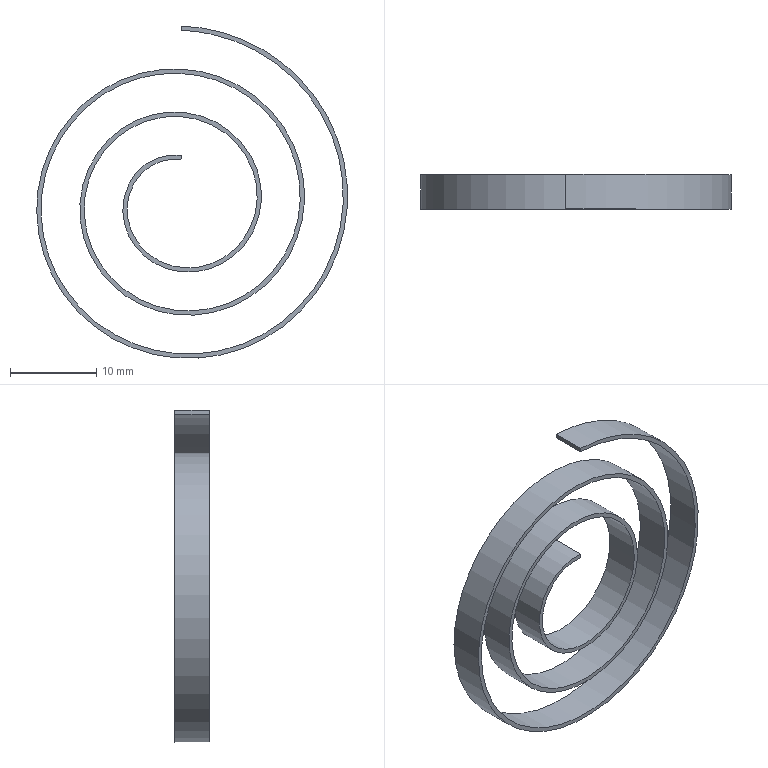Part | SolidWorks | features Helix 1, Sweep 1 | 1 solid | 6 faces | box 36.034 x 4 x 38.516 mm | volume 481.288 mm3 | plane 4 | spline 2